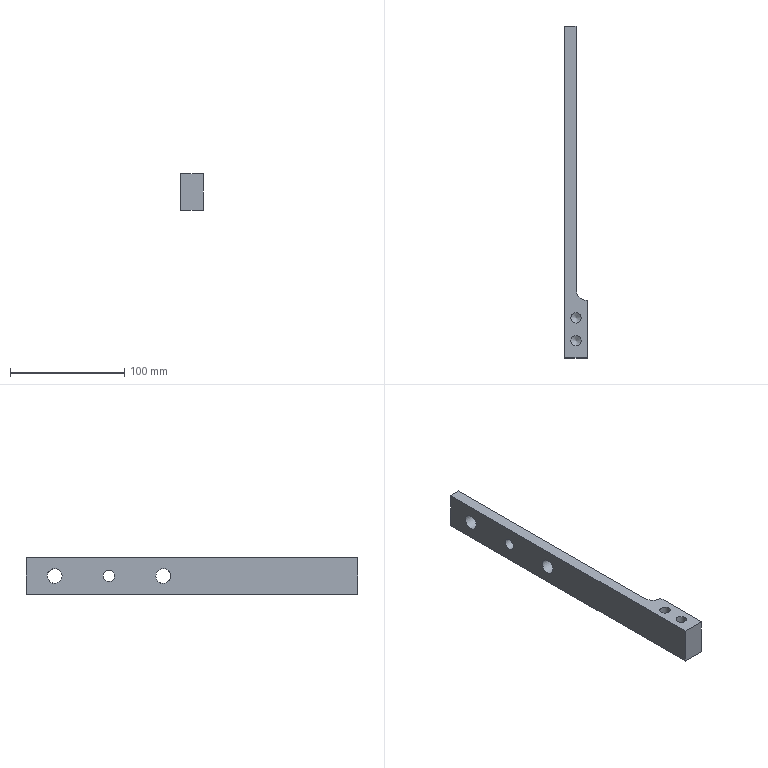Part | NX | features solid 2 | 1 solid | 15 faces | box 20 x 290 x 32 mm | volume 102624 mm3 | plane 7 | cylinder 6 | cone 2 | commonest cylinder face diameters 9 x2 13 x2 10 x1 20 x1
STEP:
#1=CARTESIAN_POINT('',(53.,515.,-95.));
#2=VERTEX_POINT('',#1);
#3=CARTESIAN_POINT('',(43.,525.,-95.));
#4=VERTEX_POINT('',#3);
#5=CARTESIAN_POINT('',(53.,525.,-95.));
#6=DIRECTION('',(0.,0.,-1.));
#7=DIRECTION('',(0.,-1.,0.));
#8=AXIS2_PLACEMENT_3D('',#5,#6,#7);
#9=CIRCLE('',#8,10.);
#10=EDGE_CURVE('',#2,#4,#9,.T.);
#11=ORIENTED_EDGE('',*,*,#10,.T.);
#12=CARTESIAN_POINT('',(43.,525.,-63.));
#13=VERTEX_POINT('',#12);
#14=CARTESIAN_POINT('',(43.,525.,-63.));
#15=DIRECTION('',(0.,0.,-1.));
#16=VECTOR('',#15,1000.);
#17=LINE('',#14,#16);
#18=EDGE_CURVE('',#13,#4,#17,.T.);
#19=ORIENTED_EDGE('',*,*,#18,.F.);
#20=CARTESIAN_POINT('',(53.,515.,-63.));
#21=VERTEX_POINT('',#20);
#22=CARTESIAN_POINT('',(53.,525.,-63.));
#23=DIRECTION('',(0.,0.,-1.));
#24=DIRECTION('',(0.,-1.,0.));
#25=AXIS2_PLACEMENT_3D('',#22,#23,#24);
#26=CIRCLE('',#25,10.);
#27=EDGE_CURVE('',#21,#13,#26,.T.);
#28=ORIENTED_EDGE('',*,*,#27,.F.);
#29=CARTESIAN_POINT('',(53.,515.,-63.));
#30=DIRECTION('',(0.,0.,-1.));
#31=VECTOR('',#30,1000.);
#32=LINE('',#29,#31);
#33=EDGE_CURVE('',#21,#2,#32,.T.);
#34=ORIENTED_EDGE('',*,*,#33,.T.);
#35=EDGE_LOOP('',(#11,#19,#28,#34));
#36=FACE_BOUND('',#35,.T.);
#37=CARTESIAN_POINT('',(53.,525.,-63.));
#38=DIRECTION('',(0.,0.,-1.));
#39=DIRECTION('',(0.,1.,0.));
#40=AXIS2_PLACEMENT_3D('',#37,#38,#39);
#41=CYLINDRICAL_SURFACE('',#40,10.);
#42=ADVANCED_FACE('',(#36),#41,.F.);
#43=CARTESIAN_POINT('',(43.,687.5,-79.));
#44=VERTEX_POINT('',#43);
#45=CARTESIAN_POINT('',(43.,682.5,-79.));
#46=DIRECTION('',(1.,0.,0.));
#47=DIRECTION('',(0.,1.,0.));
#48=AXIS2_PLACEMENT_3D('',#45,#46,#47);
#49=CIRCLE('',#48,5.);
#50=EDGE_CURVE('',#44,#44,#49,.T.);
#51=ORIENTED_EDGE('',*,*,#50,.F.);
#52=EDGE_LOOP('',(#51));
#53=FACE_BOUND('',#52,.T.);
#54=CARTESIAN_POINT('',(43.,641.5,-79.));
#55=VERTEX_POINT('',#54);
#56=CARTESIAN_POINT('',(43.,635.,-79.));
#57=DIRECTION('',(1.,0.,0.));
#58=DIRECTION('',(0.,1.,0.));
#59=AXIS2_PLACEMENT_3D('',#56,#57,#58);
#60=CIRCLE('',#59,6.5);
#61=EDGE_CURVE('',#55,#55,#60,.T.);
#62=ORIENTED_EDGE('',*,*,#61,.F.);
#63=EDGE_LOOP('',(#62));
#64=FACE_BOUND('',#63,.T.);
#65=CARTESIAN_POINT('',(43.,736.5,-79.));
#66=VERTEX_POINT('',#65);
#67=CARTESIAN_POINT('',(43.,730.,-79.));
#68=DIRECTION('',(1.,0.,0.));
#69=DIRECTION('',(0.,1.,0.));
#70=AXIS2_PLACEMENT_3D('',#67,#68,#69);
#71=CIRCLE('',#70,6.5);
#72=EDGE_CURVE('',#66,#66,#71,.T.);
#73=ORIENTED_EDGE('',*,*,#72,.F.);
#74=EDGE_LOOP('',(#73));
#75=FACE_BOUND('',#74,.T.);
#76=CARTESIAN_POINT('',(43.,755.,-95.));
#77=VERTEX_POINT('',#76);
#78=CARTESIAN_POINT('',(43.,525.,-95.));
#79=DIRECTION('',(0.,1.,0.));
#80=VECTOR('',#79,1000.);
#81=LINE('',#78,#80);
#82=EDGE_CURVE('',#4,#77,#81,.T.);
#83=ORIENTED_EDGE('',*,*,#82,.T.);
#84=CARTESIAN_POINT('',(43.,755.,-63.));
#85=VERTEX_POINT('',#84);
#86=CARTESIAN_POINT('',(43.,755.,-63.));
#87=DIRECTION('',(0.,0.,-1.));
#88=VECTOR('',#87,1000.);
#89=LINE('',#86,#88);
#90=EDGE_CURVE('',#85,#77,#89,.T.);
#91=ORIENTED_EDGE('',*,*,#90,.F.);
#92=CARTESIAN_POINT('',(43.,525.,-63.));
#93=DIRECTION('',(0.,1.,0.));
#94=VECTOR('',#93,1000.);
#95=LINE('',#92,#94);
#96=EDGE_CURVE('',#13,#85,#95,.T.);
#97=ORIENTED_EDGE('',*,*,#96,.F.);
#98=ORIENTED_EDGE('',*,*,#18,.T.);
#99=EDGE_LOOP('',(#83,#91,#97,#98));
#100=FACE_BOUND('',#99,.T.);
#101=CARTESIAN_POINT('',(43.,525.,-63.));
#102=DIRECTION('',(1.,0.,0.));
#103=DIRECTION('',(0.,-1.,0.));
#104=AXIS2_PLACEMENT_3D('',#101,#102,#103);
#105=PLANE('',#104);
#106=ADVANCED_FACE('',(#53,#64,#75,#100),#105,.T.);
#107=CARTESIAN_POINT('',(33.,755.,-95.));
#108=VERTEX_POINT('',#107);
#109=CARTESIAN_POINT('',(53.,755.,-95.));
#110=DIRECTION('',(-1.,0.,0.));
#111=VECTOR('',#110,1000.);
#112=LINE('',#109,#111);
#113=EDGE_CURVE('',#77,#108,#112,.T.);
#114=ORIENTED_EDGE('',*,*,#113,.T.);
#115=CARTESIAN_POINT('',(33.,755.,-63.));
#116=VERTEX_POINT('',#115);
#117=CARTESIAN_POINT('',(33.,755.,-63.));
#118=DIRECTION('',(0.,0.,-1.));
#119=VECTOR('',#118,1000.);
#120=LINE('',#117,#119);
#121=EDGE_CURVE('',#116,#108,#120,.T.);
#122=ORIENTED_EDGE('',*,*,#121,.F.);
#123=CARTESIAN_POINT('',(53.,755.,-63.));
#124=DIRECTION('',(-1.,0.,0.));
#125=VECTOR('',#124,1000.);
#126=LINE('',#123,#125);
#127=EDGE_CURVE('',#85,#116,#126,.T.);
#128=ORIENTED_EDGE('',*,*,#127,.F.);
#129=ORIENTED_EDGE('',*,*,#90,.T.);
#130=EDGE_LOOP('',(#114,#122,#128,#129));
#131=FACE_BOUND('',#130,.T.);
#132=CARTESIAN_POINT('',(43.,755.,-63.));
#133=DIRECTION('',(0.,1.,0.));
#134=DIRECTION('',(0.,0.,1.));
#135=AXIS2_PLACEMENT_3D('',#132,#133,#134);
#136=PLANE('',#135);
#137=ADVANCED_FACE('',(#131),#136,.T.);
#138=CARTESIAN_POINT('',(33.,682.5,-74.));
#139=VERTEX_POINT('',#138);
#140=CARTESIAN_POINT('',(33.,682.5,-79.));
#141=DIRECTION('',(-1.,0.,0.));
#142=DIRECTION('',(0.,0.,1.));
#143=AXIS2_PLACEMENT_3D('',#140,#141,#142);
#144=CIRCLE('',#143,5.);
#145=EDGE_CURVE('',#139,#139,#144,.F.);
#146=ORIENTED_EDGE('',*,*,#145,.T.);
#147=EDGE_LOOP('',(#146));
#148=FACE_BOUND('',#147,.T.);
#149=CARTESIAN_POINT('',(33.,635.,-72.5));
#150=VERTEX_POINT('',#149);
#151=CARTESIAN_POINT('',(33.,635.,-79.));
#152=DIRECTION('',(-1.,0.,0.));
#153=DIRECTION('',(0.,0.,1.));
#154=AXIS2_PLACEMENT_3D('',#151,#152,#153);
#155=CIRCLE('',#154,6.5);
#156=EDGE_CURVE('',#150,#150,#155,.F.);
#157=ORIENTED_EDGE('',*,*,#156,.T.);
#158=EDGE_LOOP('',(#157));
#159=FACE_BOUND('',#158,.T.);
#160=CARTESIAN_POINT('',(33.,730.,-72.5));
#161=VERTEX_POINT('',#160);
#162=CARTESIAN_POINT('',(33.,730.,-79.));
#163=DIRECTION('',(-1.,0.,0.));
#164=DIRECTION('',(0.,0.,1.));
#165=AXIS2_PLACEMENT_3D('',#162,#163,#164);
#166=CIRCLE('',#165,6.5);
#167=EDGE_CURVE('',#161,#161,#166,.F.);
#168=ORIENTED_EDGE('',*,*,#167,.T.);
#169=EDGE_LOOP('',(#168));
#170=FACE_BOUND('',#169,.T.);
#171=CARTESIAN_POINT('',(33.,465.,-95.));
#172=VERTEX_POINT('',#171);
#173=CARTESIAN_POINT('',(33.,745.,-95.));
#174=DIRECTION('',(0.,-1.,0.));
#175=VECTOR('',#174,1000.);
#176=LINE('',#173,#175);
#177=EDGE_CURVE('',#108,#172,#176,.T.);
#178=ORIENTED_EDGE('',*,*,#177,.T.);
#179=CARTESIAN_POINT('',(33.,465.,-63.));
#180=VERTEX_POINT('',#179);
#181=CARTESIAN_POINT('',(33.,465.,-63.));
#182=DIRECTION('',(0.,0.,-1.));
#183=VECTOR('',#182,1000.);
#184=LINE('',#181,#183);
#185=EDGE_CURVE('',#180,#172,#184,.T.);
#186=ORIENTED_EDGE('',*,*,#185,.F.);
#187=CARTESIAN_POINT('',(33.,745.,-63.));
#188=DIRECTION('',(0.,-1.,0.));
#189=VECTOR('',#188,1000.);
#190=LINE('',#187,#189);
#191=EDGE_CURVE('',#116,#180,#190,.T.);
#192=ORIENTED_EDGE('',*,*,#191,.F.);
#193=ORIENTED_EDGE('',*,*,#121,.T.);
#194=EDGE_LOOP('',(#178,#186,#192,#193));
#195=FACE_BOUND('',#194,.T.);
#196=CARTESIAN_POINT('',(33.,745.,-63.));
#197=DIRECTION('',(-1.,0.,0.));
#198=DIRECTION('',(0.,0.,1.));
#199=AXIS2_PLACEMENT_3D('',#196,#197,#198);
#200=PLANE('',#199);
#201=ADVANCED_FACE('',(#148,#159,#170,#195),#200,.T.);
#202=CARTESIAN_POINT('',(53.,465.,-95.));
#203=VERTEX_POINT('',#202);
#204=CARTESIAN_POINT('',(33.,465.,-95.));
#205=DIRECTION('',(1.,0.,0.));
#206=VECTOR('',#205,1000.);
#207=LINE('',#204,#206);
#208=EDGE_CURVE('',#172,#203,#207,.T.);
#209=ORIENTED_EDGE('',*,*,#208,.T.);
#210=CARTESIAN_POINT('',(53.,465.,-63.));
#211=VERTEX_POINT('',#210);
#212=CARTESIAN_POINT('',(53.,465.,-63.));
#213=DIRECTION('',(0.,0.,-1.));
#214=VECTOR('',#213,1000.);
#215=LINE('',#212,#214);
#216=EDGE_CURVE('',#211,#203,#215,.T.);
#217=ORIENTED_EDGE('',*,*,#216,.F.);
#218=CARTESIAN_POINT('',(33.,465.,-63.));
#219=DIRECTION('',(1.,0.,0.));
#220=VECTOR('',#219,1000.);
#221=LINE('',#218,#220);
#222=EDGE_CURVE('',#180,#211,#221,.T.);
#223=ORIENTED_EDGE('',*,*,#222,.F.);
#224=ORIENTED_EDGE('',*,*,#185,.T.);
#225=EDGE_LOOP('',(#209,#217,#223,#224));
#226=FACE_BOUND('',#225,.T.);
#227=CARTESIAN_POINT('',(33.,465.,-63.));
#228=DIRECTION('',(0.,-1.,0.));
#229=DIRECTION('',(0.,0.,-1.));
#230=AXIS2_PLACEMENT_3D('',#227,#228,#229);
#231=PLANE('',#230);
#232=ADVANCED_FACE('',(#226),#231,.T.);
#233=CARTESIAN_POINT('',(53.,465.,-95.));
#234=DIRECTION('',(0.,1.,0.));
#235=VECTOR('',#234,1000.);
#236=LINE('',#233,#235);
#237=EDGE_CURVE('',#203,#2,#236,.T.);
#238=ORIENTED_EDGE('',*,*,#237,.T.);
#239=ORIENTED_EDGE('',*,*,#33,.F.);
#240=CARTESIAN_POINT('',(53.,465.,-63.));
#241=DIRECTION('',(0.,1.,0.));
#242=VECTOR('',#241,1000.);
#243=LINE('',#240,#242);
#244=EDGE_CURVE('',#211,#21,#243,.T.);
#245=ORIENTED_EDGE('',*,*,#244,.F.);
#246=ORIENTED_EDGE('',*,*,#216,.T.);
#247=EDGE_LOOP('',(#238,#239,#245,#246));
#248=FACE_BOUND('',#247,.T.);
#249=CARTESIAN_POINT('',(53.,465.,-63.));
#250=DIRECTION('',(1.,0.,0.));
#251=DIRECTION('',(0.,0.,-1.));
#252=AXIS2_PLACEMENT_3D('',#249,#250,#251);
#253=PLANE('',#252);
#254=ADVANCED_FACE('',(#248),#253,.T.);
#255=CARTESIAN_POINT('',(43.,504.5,-63.));
#256=VERTEX_POINT('',#255);
#257=CARTESIAN_POINT('',(43.,500.,-63.));
#258=DIRECTION('',(0.,0.,1.));
#259=DIRECTION('',(0.,1.,0.));
#260=AXIS2_PLACEMENT_3D('',#257,#258,#259);
#261=CIRCLE('',#260,4.5);
#262=EDGE_CURVE('',#256,#256,#261,.T.);
#263=ORIENTED_EDGE('',*,*,#262,.F.);
#264=EDGE_LOOP('',(#263));
#265=FACE_BOUND('',#264,.T.);
#266=CARTESIAN_POINT('',(43.,484.5,-63.));
#267=VERTEX_POINT('',#266);
#268=CARTESIAN_POINT('',(43.,480.,-63.));
#269=DIRECTION('',(0.,0.,1.));
#270=DIRECTION('',(0.,1.,0.));
#271=AXIS2_PLACEMENT_3D('',#268,#269,#270);
#272=CIRCLE('',#271,4.5);
#273=EDGE_CURVE('',#267,#267,#272,.T.);
#274=ORIENTED_EDGE('',*,*,#273,.F.);
#275=EDGE_LOOP('',(#274));
#276=FACE_BOUND('',#275,.T.);
#277=ORIENTED_EDGE('',*,*,#27,.T.);
#278=ORIENTED_EDGE('',*,*,#96,.T.);
#279=ORIENTED_EDGE('',*,*,#127,.T.);
#280=ORIENTED_EDGE('',*,*,#191,.T.);
#281=ORIENTED_EDGE('',*,*,#222,.T.);
#282=ORIENTED_EDGE('',*,*,#244,.T.);
#283=EDGE_LOOP('',(#277,#278,#279,#280,#281,#282));
#284=FACE_BOUND('',#283,.T.);
#285=CARTESIAN_POINT('',(53.,525.,-63.));
#286=DIRECTION('',(0.,0.,1.));
#287=DIRECTION('',(0.,-1.,0.));
#288=AXIS2_PLACEMENT_3D('',#285,#286,#287);
#289=PLANE('',#288);
#290=ADVANCED_FACE('',(#265,#276,#284),#289,.T.);
#291=ORIENTED_EDGE('',*,*,#10,.F.);
#292=ORIENTED_EDGE('',*,*,#237,.F.);
#293=ORIENTED_EDGE('',*,*,#208,.F.);
#294=ORIENTED_EDGE('',*,*,#177,.F.);
#295=ORIENTED_EDGE('',*,*,#113,.F.);
#296=ORIENTED_EDGE('',*,*,#82,.F.);
#297=EDGE_LOOP('',(#291,#292,#293,#294,#295,#296));
#298=FACE_BOUND('',#297,.T.);
#299=CARTESIAN_POINT('',(53.,525.,-95.));
#300=DIRECTION('',(0.,0.,1.));
#301=DIRECTION('',(0.,-1.,0.));
#302=AXIS2_PLACEMENT_3D('',#299,#300,#301);
#303=PLANE('',#302);
#304=ADVANCED_FACE('',(#298),#303,.F.);
#305=ORIENTED_EDGE('',*,*,#167,.F.);
#306=EDGE_LOOP('',(#305));
#307=FACE_BOUND('',#306,.T.);
#308=ORIENTED_EDGE('',*,*,#72,.T.);
#309=EDGE_LOOP('',(#308));
#310=FACE_BOUND('',#309,.T.);
#311=CARTESIAN_POINT('',(43.,730.,-79.));
#312=DIRECTION('',(-1.,0.,0.));
#313=DIRECTION('',(0.,1.,0.));
#314=AXIS2_PLACEMENT_3D('',#311,#312,#313);
#315=CYLINDRICAL_SURFACE('',#314,6.5);
#316=ADVANCED_FACE('',(#307,#310),#315,.F.);
#317=ORIENTED_EDGE('',*,*,#156,.F.);
#318=EDGE_LOOP('',(#317));
#319=FACE_BOUND('',#318,.T.);
#320=ORIENTED_EDGE('',*,*,#61,.T.);
#321=EDGE_LOOP('',(#320));
#322=FACE_BOUND('',#321,.T.);
#323=CARTESIAN_POINT('',(43.,635.,-79.));
#324=DIRECTION('',(-1.,0.,0.));
#325=DIRECTION('',(0.,1.,0.));
#326=AXIS2_PLACEMENT_3D('',#323,#324,#325);
#327=CYLINDRICAL_SURFACE('',#326,6.5);
#328=ADVANCED_FACE('',(#319,#322),#327,.F.);
#329=CARTESIAN_POINT('',(43.,484.5,-89.));
#330=VERTEX_POINT('',#329);
#331=CARTESIAN_POINT('',(43.,480.,-89.));
#332=DIRECTION('',(0.,0.,1.));
#333=DIRECTION('',(0.,1.,0.));
#334=AXIS2_PLACEMENT_3D('',#331,#332,#333);
#335=CIRCLE('',#334,4.5);
#336=EDGE_CURVE('',#330,#330,#335,.T.);
#337=ORIENTED_EDGE('',*,*,#336,.T.);
#338=EDGE_LOOP('',(#337));
#339=FACE_BOUND('',#338,.T.);
#340=CARTESIAN_POINT('',(43.,480.,-91.704));
#341=VERTEX_POINT('',#340);
#342=VERTEX_LOOP('',#341);
#343=FACE_BOUND('',#342,.T.);
#344=CARTESIAN_POINT('',(43.,480.,-89.));
#345=DIRECTION('',(0.,0.,1.));
#346=DIRECTION('',(0.,-1.,0.));
#347=AXIS2_PLACEMENT_3D('',#344,#345,#346);
#348=CONICAL_SURFACE('',#347,4.5,1.03);
#349=ADVANCED_FACE('',(#339,#343),#348,.F.);
#350=ORIENTED_EDGE('',*,*,#336,.F.);
#351=EDGE_LOOP('',(#350));
#352=FACE_BOUND('',#351,.T.);
#353=ORIENTED_EDGE('',*,*,#273,.T.);
#354=EDGE_LOOP('',(#353));
#355=FACE_BOUND('',#354,.T.);
#356=CARTESIAN_POINT('',(43.,480.,-63.));
#357=DIRECTION('',(0.,0.,-1.));
#358=DIRECTION('',(0.,1.,0.));
#359=AXIS2_PLACEMENT_3D('',#356,#357,#358);
#360=CYLINDRICAL_SURFACE('',#359,4.5);
#361=ADVANCED_FACE('',(#352,#355),#360,.F.);
#362=CARTESIAN_POINT('',(43.,504.5,-89.));
#363=VERTEX_POINT('',#362);
#364=CARTESIAN_POINT('',(43.,500.,-89.));
#365=DIRECTION('',(0.,0.,1.));
#366=DIRECTION('',(0.,1.,0.));
#367=AXIS2_PLACEMENT_3D('',#364,#365,#366);
#368=CIRCLE('',#367,4.5);
#369=EDGE_CURVE('',#363,#363,#368,.T.);
#370=ORIENTED_EDGE('',*,*,#369,.T.);
#371=EDGE_LOOP('',(#370));
#372=FACE_BOUND('',#371,.T.);
#373=CARTESIAN_POINT('',(43.,500.,-91.704));
#374=VERTEX_POINT('',#373);
#375=VERTEX_LOOP('',#374);
#376=FACE_BOUND('',#375,.T.);
#377=CARTESIAN_POINT('',(43.,500.,-89.));
#378=DIRECTION('',(0.,0.,1.));
#379=DIRECTION('',(0.,-1.,0.));
#380=AXIS2_PLACEMENT_3D('',#377,#378,#379);
#381=CONICAL_SURFACE('',#380,4.5,1.03);
#382=ADVANCED_FACE('',(#372,#376),#381,.F.);
#383=ORIENTED_EDGE('',*,*,#369,.F.);
#384=EDGE_LOOP('',(#383));
#385=FACE_BOUND('',#384,.T.);
#386=ORIENTED_EDGE('',*,*,#262,.T.);
#387=EDGE_LOOP('',(#386));
#388=FACE_BOUND('',#387,.T.);
#389=CARTESIAN_POINT('',(43.,500.,-63.));
#390=DIRECTION('',(0.,0.,-1.));
#391=DIRECTION('',(0.,1.,0.));
#392=AXIS2_PLACEMENT_3D('',#389,#390,#391);
#393=CYLINDRICAL_SURFACE('',#392,4.5);
#394=ADVANCED_FACE('',(#385,#388),#393,.F.);
#395=ORIENTED_EDGE('',*,*,#145,.F.);
#396=EDGE_LOOP('',(#395));
#397=FACE_BOUND('',#396,.T.);
#398=ORIENTED_EDGE('',*,*,#50,.T.);
#399=EDGE_LOOP('',(#398));
#400=FACE_BOUND('',#399,.T.);
#401=CARTESIAN_POINT('',(43.,682.5,-79.));
#402=DIRECTION('',(-1.,0.,0.));
#403=DIRECTION('',(0.,1.,0.));
#404=AXIS2_PLACEMENT_3D('',#401,#402,#403);
#405=CYLINDRICAL_SURFACE('',#404,5.);
#406=ADVANCED_FACE('',(#397,#400),#405,.F.);
#407=CLOSED_SHELL('',(#42,#106,#137,#201,#232,#254,#290,#304,#316,#328,#349,#361,#382,#394,#406));
#408=MANIFOLD_SOLID_BREP('',#407);
#409=(LENGTH_UNIT()NAMED_UNIT(*)SI_UNIT(.MILLI.,.METRE.));
#410=UNCERTAINTY_MEASURE_WITH_UNIT(LENGTH_MEASURE(0.00001),#409,'','');
#411=(NAMED_UNIT(*)PLANE_ANGLE_UNIT()SI_UNIT($,.RADIAN.));
#412=(NAMED_UNIT(*)SI_UNIT($,.STERADIAN.)SOLID_ANGLE_UNIT());
#413=(GEOMETRIC_REPRESENTATION_CONTEXT(3)GLOBAL_UNCERTAINTY_ASSIGNED_CONTEXT((#410))GLOBAL_UNIT_ASSIGNED_CONTEXT((#409,#411,#412))REPRESENTATION_CONTEXT('',''));
#414=ADVANCED_BREP_SHAPE_REPRESENTATION('',(#408),#413);